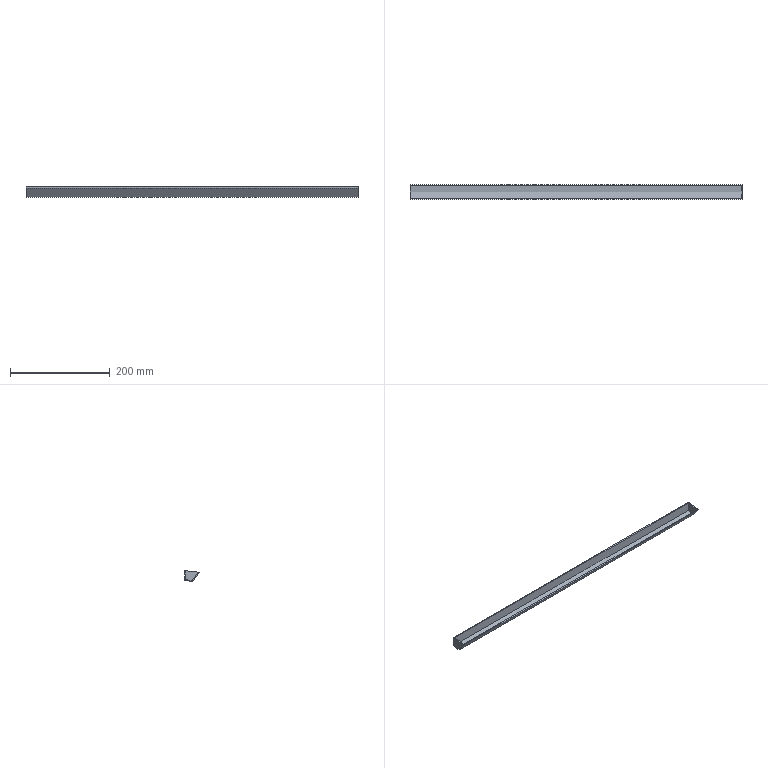Part | SolidWorks | features ICE 2, Extrusion 1 | 1 solid | 11 faces | box 665 x 29.785 x 21.93 mm | volume 75134 mm3 | plane 11
STEP:
#1=CARTESIAN_POINT('',(0.,-2.,1.774));
#2=VERTEX_POINT('',#1);
#3=CARTESIAN_POINT('',(0.,-2.,19.759));
#4=VERTEX_POINT('',#3);
#5=CARTESIAN_POINT('',(0.,-2.,1.774));
#6=DIRECTION('',(0.,0.,1.));
#7=VECTOR('',#6,1000.);
#8=LINE('',#5,#7);
#9=EDGE_CURVE('',#2,#4,#8,.T.);
#10=ORIENTED_EDGE('',*,*,#9,.F.);
#11=CARTESIAN_POINT('',(0.,-15.122,0.1939));
#12=VERTEX_POINT('',#11);
#13=CARTESIAN_POINT('',(0.,-15.122,0.1939));
#14=DIRECTION('',(0.,0.9928,0.1195));
#15=VECTOR('',#14,1000.);
#16=LINE('',#13,#15);
#17=EDGE_CURVE('',#12,#2,#16,.T.);
#18=ORIENTED_EDGE('',*,*,#17,.F.);
#19=CARTESIAN_POINT('',(0.,-27.492,16.69));
#20=VERTEX_POINT('',#19);
#21=CARTESIAN_POINT('',(0.,-27.492,16.69));
#22=DIRECTION('',(0.,0.5999,-0.8001));
#23=VECTOR('',#22,1000.);
#24=LINE('',#21,#23);
#25=EDGE_CURVE('',#20,#12,#24,.T.);
#26=ORIENTED_EDGE('',*,*,#25,.F.);
#27=CARTESIAN_POINT('',(0.,0.,20.));
#28=DIRECTION('',(0.,-0.9928,-0.1195));
#29=VECTOR('',#28,1000.);
#30=LINE('',#27,#29);
#31=EDGE_CURVE('',#4,#20,#30,.T.);
#32=ORIENTED_EDGE('',*,*,#31,.F.);
#33=EDGE_LOOP('',(#10,#18,#26,#32));
#34=FACE_OUTER_BOUND('',#33,.T.);
#35=CARTESIAN_POINT('',(0.,0.,0.));
#36=DIRECTION('',(1.,0.,0.));
#37=DIRECTION('',(0.,0.,-1.));
#38=AXIS2_PLACEMENT_3D('',#35,#36,#37);
#39=PLANE('',#38);
#40=ADVANCED_FACE('',(#34),#39,.F.);
#41=CARTESIAN_POINT('',(2.,-16.03,-1.93));
#42=VERTEX_POINT('',#41);
#43=CARTESIAN_POINT('',(-663.,-16.03,-1.93));
#44=VERTEX_POINT('',#43);
#45=CARTESIAN_POINT('',(2.,-16.03,-1.93));
#46=DIRECTION('',(-1.,0.,0.));
#47=VECTOR('',#46,1000.);
#48=LINE('',#45,#47);
#49=EDGE_CURVE('',#42,#44,#48,.T.);
#50=ORIENTED_EDGE('',*,*,#49,.T.);
#51=CARTESIAN_POINT('',(-663.,0.,0.));
#52=VERTEX_POINT('',#51);
#53=CARTESIAN_POINT('',(-663.,0.,0.));
#54=DIRECTION('',(0.,-0.9928,-0.1195));
#55=VECTOR('',#54,1000.);
#56=LINE('',#53,#55);
#57=EDGE_CURVE('',#52,#44,#56,.T.);
#58=ORIENTED_EDGE('',*,*,#57,.F.);
#59=CARTESIAN_POINT('',(2.,0.,0.));
#60=VERTEX_POINT('',#59);
#61=CARTESIAN_POINT('',(2.,0.,0.));
#62=DIRECTION('',(-1.,0.,0.));
#63=VECTOR('',#62,1000.);
#64=LINE('',#61,#63);
#65=EDGE_CURVE('',#60,#52,#64,.T.);
#66=ORIENTED_EDGE('',*,*,#65,.F.);
#67=CARTESIAN_POINT('',(2.,-16.03,-1.93));
#68=DIRECTION('',(0.,0.9928,0.1195));
#69=VECTOR('',#68,1000.);
#70=LINE('',#67,#69);
#71=EDGE_CURVE('',#42,#60,#70,.T.);
#72=ORIENTED_EDGE('',*,*,#71,.F.);
#73=EDGE_LOOP('',(#50,#58,#66,#72));
#74=FACE_OUTER_BOUND('',#73,.T.);
#75=CARTESIAN_POINT('',(2.,-16.03,-1.93));
#76=DIRECTION('',(0.,-0.1195,0.9928));
#77=DIRECTION('',(0.,-0.9928,-0.1195));
#78=AXIS2_PLACEMENT_3D('',#75,#76,#77);
#79=PLANE('',#78);
#80=ADVANCED_FACE('',(#74),#79,.F.);
#81=ORIENTED_EDGE('',*,*,#65,.T.);
#82=CARTESIAN_POINT('',(-663.,0.,20.));
#83=VERTEX_POINT('',#82);
#84=CARTESIAN_POINT('',(-663.,0.,20.));
#85=DIRECTION('',(0.,0.,-1.));
#86=VECTOR('',#85,1000.);
#87=LINE('',#84,#86);
#88=EDGE_CURVE('',#83,#52,#87,.T.);
#89=ORIENTED_EDGE('',*,*,#88,.F.);
#90=CARTESIAN_POINT('',(2.,0.,20.));
#91=VERTEX_POINT('',#90);
#92=CARTESIAN_POINT('',(2.,0.,20.));
#93=DIRECTION('',(-1.,0.,0.));
#94=VECTOR('',#93,1000.);
#95=LINE('',#92,#94);
#96=EDGE_CURVE('',#91,#83,#95,.T.);
#97=ORIENTED_EDGE('',*,*,#96,.F.);
#98=CARTESIAN_POINT('',(2.,0.,0.));
#99=DIRECTION('',(0.,0.,1.));
#100=VECTOR('',#99,1000.);
#101=LINE('',#98,#100);
#102=EDGE_CURVE('',#60,#91,#101,.T.);
#103=ORIENTED_EDGE('',*,*,#102,.F.);
#104=EDGE_LOOP('',(#81,#89,#97,#103));
#105=FACE_OUTER_BOUND('',#104,.T.);
#106=CARTESIAN_POINT('',(2.,0.,0.));
#107=DIRECTION('',(0.,-1.,0.));
#108=DIRECTION('',(0.,0.,-1.));
#109=AXIS2_PLACEMENT_3D('',#106,#107,#108);
#110=PLANE('',#109);
#111=ADVANCED_FACE('',(#105),#110,.F.);
#112=CARTESIAN_POINT('',(-661.,-27.492,16.69));
#113=VERTEX_POINT('',#112);
#114=CARTESIAN_POINT('',(-661.,-27.492,16.69));
#115=DIRECTION('',(1.,0.,0.));
#116=VECTOR('',#115,1000.);
#117=LINE('',#114,#116);
#118=EDGE_CURVE('',#113,#20,#117,.T.);
#119=ORIENTED_EDGE('',*,*,#118,.F.);
#120=CARTESIAN_POINT('',(-661.,-2.,19.759));
#121=VERTEX_POINT('',#120);
#122=CARTESIAN_POINT('',(-661.,-29.785,16.414));
#123=DIRECTION('',(0.,0.9928,0.1195));
#124=VECTOR('',#123,1000.);
#125=LINE('',#122,#124);
#126=EDGE_CURVE('',#113,#121,#125,.T.);
#127=ORIENTED_EDGE('',*,*,#126,.T.);
#128=CARTESIAN_POINT('',(-661.,-2.,19.759));
#129=DIRECTION('',(1.,0.,0.));
#130=VECTOR('',#129,1000.);
#131=LINE('',#128,#130);
#132=EDGE_CURVE('',#121,#4,#131,.T.);
#133=ORIENTED_EDGE('',*,*,#132,.T.);
#134=ORIENTED_EDGE('',*,*,#31,.T.);
#135=EDGE_LOOP('',(#119,#127,#133,#134));
#136=FACE_BOUND('',#135,.T.);
#137=ORIENTED_EDGE('',*,*,#96,.T.);
#138=CARTESIAN_POINT('',(-663.,-29.785,16.414));
#139=VERTEX_POINT('',#138);
#140=CARTESIAN_POINT('',(-663.,-29.785,16.414));
#141=DIRECTION('',(0.,0.9928,0.1195));
#142=VECTOR('',#141,1000.);
#143=LINE('',#140,#142);
#144=EDGE_CURVE('',#139,#83,#143,.T.);
#145=ORIENTED_EDGE('',*,*,#144,.F.);
#146=CARTESIAN_POINT('',(2.,-29.785,16.414));
#147=VERTEX_POINT('',#146);
#148=CARTESIAN_POINT('',(2.,-29.785,16.414));
#149=DIRECTION('',(-1.,0.,0.));
#150=VECTOR('',#149,1000.);
#151=LINE('',#148,#150);
#152=EDGE_CURVE('',#147,#139,#151,.T.);
#153=ORIENTED_EDGE('',*,*,#152,.F.);
#154=CARTESIAN_POINT('',(2.,0.,20.));
#155=DIRECTION('',(0.,-0.9928,-0.1195));
#156=VECTOR('',#155,1000.);
#157=LINE('',#154,#156);
#158=EDGE_CURVE('',#91,#147,#157,.T.);
#159=ORIENTED_EDGE('',*,*,#158,.F.);
#160=EDGE_LOOP('',(#137,#145,#153,#159));
#161=FACE_OUTER_BOUND('',#160,.T.);
#162=CARTESIAN_POINT('',(2.,0.,20.));
#163=DIRECTION('',(0.,0.1195,-0.9928));
#164=DIRECTION('',(0.,0.9928,0.1195));
#165=AXIS2_PLACEMENT_3D('',#162,#163,#164);
#166=PLANE('',#165);
#167=ADVANCED_FACE('',(#136,#161),#166,.F.);
#168=ORIENTED_EDGE('',*,*,#152,.T.);
#169=CARTESIAN_POINT('',(-663.,-16.03,-1.93));
#170=DIRECTION('',(0.,-0.5999,0.8001));
#171=VECTOR('',#170,1000.);
#172=LINE('',#169,#171);
#173=EDGE_CURVE('',#44,#139,#172,.T.);
#174=ORIENTED_EDGE('',*,*,#173,.F.);
#175=ORIENTED_EDGE('',*,*,#49,.F.);
#176=CARTESIAN_POINT('',(2.,-29.785,16.414));
#177=DIRECTION('',(0.,0.5999,-0.8001));
#178=VECTOR('',#177,1000.);
#179=LINE('',#176,#178);
#180=EDGE_CURVE('',#147,#42,#179,.T.);
#181=ORIENTED_EDGE('',*,*,#180,.F.);
#182=EDGE_LOOP('',(#168,#174,#175,#181));
#183=FACE_OUTER_BOUND('',#182,.T.);
#184=CARTESIAN_POINT('',(2.,-29.785,16.414));
#185=DIRECTION('',(0.,0.8001,0.5999));
#186=DIRECTION('',(0.,-0.5999,0.8001));
#187=AXIS2_PLACEMENT_3D('',#184,#185,#186);
#188=PLANE('',#187);
#189=ADVANCED_FACE('',(#183),#188,.F.);
#190=ORIENTED_EDGE('',*,*,#71,.T.);
#191=ORIENTED_EDGE('',*,*,#102,.T.);
#192=ORIENTED_EDGE('',*,*,#158,.T.);
#193=ORIENTED_EDGE('',*,*,#180,.T.);
#194=EDGE_LOOP('',(#190,#191,#192,#193));
#195=FACE_OUTER_BOUND('',#194,.T.);
#196=CARTESIAN_POINT('',(2.,0.,0.));
#197=DIRECTION('',(1.,0.,0.));
#198=DIRECTION('',(0.,0.,-1.));
#199=AXIS2_PLACEMENT_3D('',#196,#197,#198);
#200=PLANE('',#199);
#201=ADVANCED_FACE('',(#195),#200,.T.);
#202=ORIENTED_EDGE('',*,*,#25,.T.);
#203=CARTESIAN_POINT('',(-661.,-15.122,0.1939));
#204=VERTEX_POINT('',#203);
#205=CARTESIAN_POINT('',(-661.,-15.122,0.1939));
#206=DIRECTION('',(1.,0.,0.));
#207=VECTOR('',#206,1000.);
#208=LINE('',#205,#207);
#209=EDGE_CURVE('',#204,#12,#208,.T.);
#210=ORIENTED_EDGE('',*,*,#209,.F.);
#211=CARTESIAN_POINT('',(-661.,-27.492,16.69));
#212=DIRECTION('',(0.,0.5999,-0.8001));
#213=VECTOR('',#212,1000.);
#214=LINE('',#211,#213);
#215=EDGE_CURVE('',#113,#204,#214,.T.);
#216=ORIENTED_EDGE('',*,*,#215,.F.);
#217=ORIENTED_EDGE('',*,*,#118,.T.);
#218=EDGE_LOOP('',(#202,#210,#216,#217));
#219=FACE_OUTER_BOUND('',#218,.T.);
#220=CARTESIAN_POINT('',(-661.,-27.492,16.69));
#221=DIRECTION('',(0.,-0.8001,-0.5999));
#222=DIRECTION('',(0.,0.5999,-0.8001));
#223=AXIS2_PLACEMENT_3D('',#220,#221,#222);
#224=PLANE('',#223);
#225=ADVANCED_FACE('',(#219),#224,.F.);
#226=ORIENTED_EDGE('',*,*,#17,.T.);
#227=CARTESIAN_POINT('',(-661.,-2.,1.774));
#228=VERTEX_POINT('',#227);
#229=CARTESIAN_POINT('',(-661.,-2.,1.774));
#230=DIRECTION('',(1.,0.,0.));
#231=VECTOR('',#230,1000.);
#232=LINE('',#229,#231);
#233=EDGE_CURVE('',#228,#2,#232,.T.);
#234=ORIENTED_EDGE('',*,*,#233,.F.);
#235=CARTESIAN_POINT('',(-661.,-15.122,0.1939));
#236=DIRECTION('',(0.,0.9928,0.1195));
#237=VECTOR('',#236,1000.);
#238=LINE('',#235,#237);
#239=EDGE_CURVE('',#204,#228,#238,.T.);
#240=ORIENTED_EDGE('',*,*,#239,.F.);
#241=ORIENTED_EDGE('',*,*,#209,.T.);
#242=EDGE_LOOP('',(#226,#234,#240,#241));
#243=FACE_OUTER_BOUND('',#242,.T.);
#244=CARTESIAN_POINT('',(-661.,-15.122,0.1939));
#245=DIRECTION('',(0.,0.1195,-0.9928));
#246=DIRECTION('',(0.,0.9928,0.1195));
#247=AXIS2_PLACEMENT_3D('',#244,#245,#246);
#248=PLANE('',#247);
#249=ADVANCED_FACE('',(#243),#248,.F.);
#250=ORIENTED_EDGE('',*,*,#9,.T.);
#251=ORIENTED_EDGE('',*,*,#132,.F.);
#252=CARTESIAN_POINT('',(-661.,-2.,1.774));
#253=DIRECTION('',(0.,0.,1.));
#254=VECTOR('',#253,1000.);
#255=LINE('',#252,#254);
#256=EDGE_CURVE('',#228,#121,#255,.T.);
#257=ORIENTED_EDGE('',*,*,#256,.F.);
#258=ORIENTED_EDGE('',*,*,#233,.T.);
#259=EDGE_LOOP('',(#250,#251,#257,#258));
#260=FACE_OUTER_BOUND('',#259,.T.);
#261=CARTESIAN_POINT('',(-661.,-2.,1.774));
#262=DIRECTION('',(0.,1.,0.));
#263=DIRECTION('',(0.,0.,1.));
#264=AXIS2_PLACEMENT_3D('',#261,#262,#263);
#265=PLANE('',#264);
#266=ADVANCED_FACE('',(#260),#265,.F.);
#267=ORIENTED_EDGE('',*,*,#57,.T.);
#268=ORIENTED_EDGE('',*,*,#173,.T.);
#269=ORIENTED_EDGE('',*,*,#144,.T.);
#270=ORIENTED_EDGE('',*,*,#88,.T.);
#271=EDGE_LOOP('',(#267,#268,#269,#270));
#272=FACE_OUTER_BOUND('',#271,.T.);
#273=CARTESIAN_POINT('',(-663.,0.,0.));
#274=DIRECTION('',(1.,0.,0.));
#275=DIRECTION('',(0.,0.,-1.));
#276=AXIS2_PLACEMENT_3D('',#273,#274,#275);
#277=PLANE('',#276);
#278=ADVANCED_FACE('',(#272),#277,.F.);
#279=ORIENTED_EDGE('',*,*,#126,.F.);
#280=ORIENTED_EDGE('',*,*,#215,.T.);
#281=ORIENTED_EDGE('',*,*,#239,.T.);
#282=ORIENTED_EDGE('',*,*,#256,.T.);
#283=EDGE_LOOP('',(#279,#280,#281,#282));
#284=FACE_OUTER_BOUND('',#283,.T.);
#285=CARTESIAN_POINT('',(-661.,0.,0.));
#286=DIRECTION('',(1.,0.,0.));
#287=DIRECTION('',(0.,0.,-1.));
#288=AXIS2_PLACEMENT_3D('',#285,#286,#287);
#289=PLANE('',#288);
#290=ADVANCED_FACE('',(#284),#289,.T.);
#291=CLOSED_SHELL('',(#40,#80,#111,#167,#189,#201,#225,#249,#266,#278,#290));
#292=MANIFOLD_SOLID_BREP('',#291);
#293=CARTESIAN_POINT('',(0.,0.,0.));
#294=DIRECTION('',(0.,0.,1.));
#295=DIRECTION('',(1.,0.,0.));
#296=AXIS2_PLACEMENT_3D('',#293,#294,#295);
#297=(LENGTH_UNIT()NAMED_UNIT(*)SI_UNIT(.MILLI.,.METRE.));
#298=UNCERTAINTY_MEASURE_WITH_UNIT(LENGTH_MEASURE(0.00001),#297,'','');
#299=(NAMED_UNIT(*)PLANE_ANGLE_UNIT()SI_UNIT($,.RADIAN.));
#300=(NAMED_UNIT(*)SI_UNIT($,.STERADIAN.)SOLID_ANGLE_UNIT());
#301=(GEOMETRIC_REPRESENTATION_CONTEXT(3)GLOBAL_UNCERTAINTY_ASSIGNED_CONTEXT((#298))GLOBAL_UNIT_ASSIGNED_CONTEXT((#297,#299,#300))REPRESENTATION_CONTEXT('',''));
#302=ADVANCED_BREP_SHAPE_REPRESENTATION('',(#292,#296),#301);